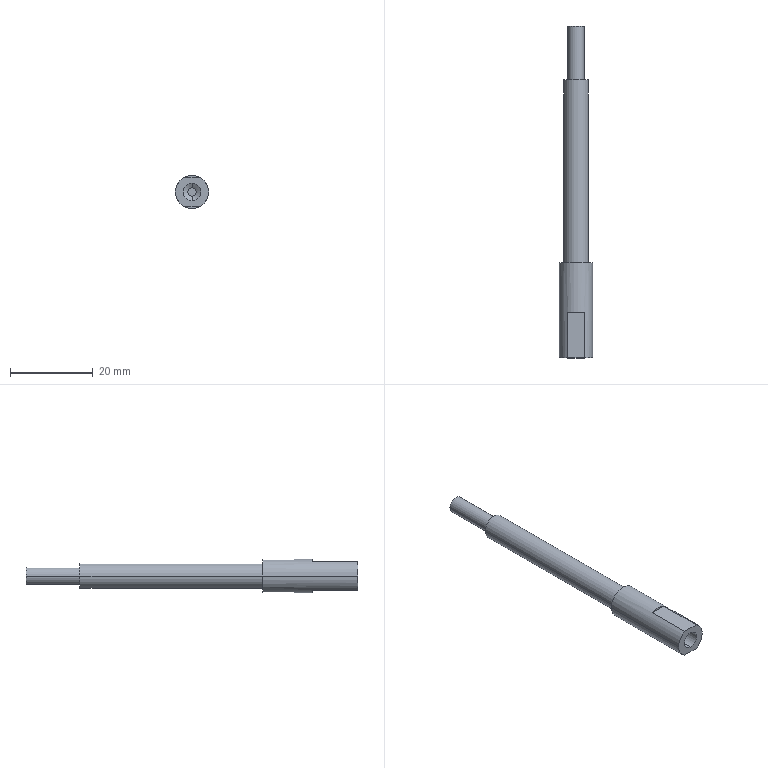Part | SolidWorks | features ICE 4, HoleWzd 1, Revolution 1 | 1 solid | 24 faces | box 8 x 80 x 8 mm | volume 2165 mm3 | cylinder 12 | plane 10 | cone 2 | commonest cylinder face diameters 2 x4 4 x2 4.2 x2 6 x2 8 x2
STEP:
#1=CARTESIAN_POINT('',(-1.,67.,0.));
#2=VERTEX_POINT('',#1);
#3=CARTESIAN_POINT('',(1.,67.,0.));
#4=VERTEX_POINT('',#3);
#5=CARTESIAN_POINT('',(0.,67.,0.));
#6=DIRECTION('',(0.,-1.,0.));
#7=DIRECTION('',(-1.,0.,0.));
#8=AXIS2_PLACEMENT_3D('',#5,#6,#7);
#9=CIRCLE('',#8,1.);
#10=EDGE_CURVE('',#2,#4,#9,.T.);
#11=ORIENTED_EDGE('',*,*,#10,.T.);
#12=CARTESIAN_POINT('',(1.,80.,0.));
#13=VERTEX_POINT('',#12);
#14=CARTESIAN_POINT('',(1.,0.,0.));
#15=DIRECTION('',(0.,1.,0.));
#16=VECTOR('',#15,1000.);
#17=LINE('',#14,#16);
#18=EDGE_CURVE('',#4,#13,#17,.T.);
#19=ORIENTED_EDGE('',*,*,#18,.T.);
#20=CARTESIAN_POINT('',(-1.,80.,0.));
#21=VERTEX_POINT('',#20);
#22=CARTESIAN_POINT('',(0.,80.,0.));
#23=DIRECTION('',(0.,1.,0.));
#24=DIRECTION('',(-1.,0.,0.));
#25=AXIS2_PLACEMENT_3D('',#22,#23,#24);
#26=CIRCLE('',#25,1.);
#27=EDGE_CURVE('',#13,#21,#26,.T.);
#28=ORIENTED_EDGE('',*,*,#27,.T.);
#29=CARTESIAN_POINT('',(-1.,0.,0.));
#30=DIRECTION('',(0.,1.,0.));
#31=VECTOR('',#30,1000.);
#32=LINE('',#29,#31);
#33=EDGE_CURVE('',#2,#21,#32,.T.);
#34=ORIENTED_EDGE('',*,*,#33,.F.);
#35=EDGE_LOOP('',(#11,#19,#28,#34));
#36=FACE_OUTER_BOUND('',#35,.T.);
#37=CARTESIAN_POINT('',(0.,0.,0.));
#38=DIRECTION('',(0.,1.,0.));
#39=DIRECTION('',(-1.,0.,0.));
#40=AXIS2_PLACEMENT_3D('',#37,#38,#39);
#41=CYLINDRICAL_SURFACE('',#40,1.);
#42=ADVANCED_FACE('',(#36),#41,.F.);
#43=CARTESIAN_POINT('',(-2.,67.,0.));
#44=VERTEX_POINT('',#43);
#45=CARTESIAN_POINT('',(2.,67.,0.));
#46=VERTEX_POINT('',#45);
#47=CARTESIAN_POINT('',(0.,67.,0.));
#48=DIRECTION('',(0.,1.,0.));
#49=DIRECTION('',(-1.,0.,0.));
#50=AXIS2_PLACEMENT_3D('',#47,#48,#49);
#51=CIRCLE('',#50,2.);
#52=EDGE_CURVE('',#44,#46,#51,.T.);
#53=ORIENTED_EDGE('',*,*,#52,.T.);
#54=CARTESIAN_POINT('',(2.,80.,0.));
#55=VERTEX_POINT('',#54);
#56=CARTESIAN_POINT('',(2.,80.,0.));
#57=DIRECTION('',(0.,1.,0.));
#58=VECTOR('',#57,1000.);
#59=LINE('',#56,#58);
#60=EDGE_CURVE('',#46,#55,#59,.T.);
#61=ORIENTED_EDGE('',*,*,#60,.T.);
#62=CARTESIAN_POINT('',(-2.,80.,0.));
#63=VERTEX_POINT('',#62);
#64=CARTESIAN_POINT('',(0.,80.,0.));
#65=DIRECTION('',(0.,1.,0.));
#66=DIRECTION('',(-1.,0.,0.));
#67=AXIS2_PLACEMENT_3D('',#64,#65,#66);
#68=CIRCLE('',#67,2.);
#69=EDGE_CURVE('',#63,#55,#68,.T.);
#70=ORIENTED_EDGE('',*,*,#69,.F.);
#71=CARTESIAN_POINT('',(-2.,80.,0.));
#72=DIRECTION('',(0.,1.,0.));
#73=VECTOR('',#72,1000.);
#74=LINE('',#71,#73);
#75=EDGE_CURVE('',#44,#63,#74,.T.);
#76=ORIENTED_EDGE('',*,*,#75,.F.);
#77=EDGE_LOOP('',(#53,#61,#70,#76));
#78=FACE_OUTER_BOUND('',#77,.T.);
#79=CARTESIAN_POINT('',(0.,80.,0.));
#80=DIRECTION('',(0.,1.,0.));
#81=DIRECTION('',(-1.,0.,0.));
#82=AXIS2_PLACEMENT_3D('',#79,#80,#81);
#83=CYLINDRICAL_SURFACE('',#82,2.);
#84=ADVANCED_FACE('',(#78),#83,.T.);
#85=CARTESIAN_POINT('',(0.,12.25,2.1));
#86=VERTEX_POINT('',#85);
#87=CARTESIAN_POINT('',(0.,12.25,-2.1));
#88=VERTEX_POINT('',#87);
#89=CARTESIAN_POINT('',(0.,12.25,0.));
#90=DIRECTION('',(0.,-1.,0.));
#91=DIRECTION('',(0.,0.,-1.));
#92=AXIS2_PLACEMENT_3D('',#89,#90,#91);
#93=CIRCLE('',#92,2.1);
#94=EDGE_CURVE('',#86,#88,#93,.T.);
#95=ORIENTED_EDGE('',*,*,#94,.F.);
#96=CARTESIAN_POINT('',(0.,0.,2.1));
#97=VERTEX_POINT('',#96);
#98=CARTESIAN_POINT('',(0.,0.,2.1));
#99=DIRECTION('',(0.,-1.,0.));
#100=VECTOR('',#99,1000.);
#101=LINE('',#98,#100);
#102=EDGE_CURVE('',#86,#97,#101,.T.);
#103=ORIENTED_EDGE('',*,*,#102,.T.);
#104=CARTESIAN_POINT('',(0.,0.,-2.1));
#105=VERTEX_POINT('',#104);
#106=CARTESIAN_POINT('',(0.,0.,0.));
#107=DIRECTION('',(0.,-1.,0.));
#108=DIRECTION('',(0.,0.,-1.));
#109=AXIS2_PLACEMENT_3D('',#106,#107,#108);
#110=CIRCLE('',#109,2.1);
#111=EDGE_CURVE('',#97,#105,#110,.T.);
#112=ORIENTED_EDGE('',*,*,#111,.T.);
#113=CARTESIAN_POINT('',(0.,0.,-2.1));
#114=DIRECTION('',(0.,-1.,0.));
#115=VECTOR('',#114,1000.);
#116=LINE('',#113,#115);
#117=EDGE_CURVE('',#88,#105,#116,.T.);
#118=ORIENTED_EDGE('',*,*,#117,.F.);
#119=EDGE_LOOP('',(#95,#103,#112,#118));
#120=FACE_OUTER_BOUND('',#119,.T.);
#121=CARTESIAN_POINT('',(0.,0.,0.));
#122=DIRECTION('',(0.,-1.,0.));
#123=DIRECTION('',(0.,0.,-1.));
#124=AXIS2_PLACEMENT_3D('',#121,#122,#123);
#125=CYLINDRICAL_SURFACE('',#124,2.1);
#126=ADVANCED_FACE('',(#120),#125,.F.);
#127=CARTESIAN_POINT('',(0.,12.911,1.));
#128=VERTEX_POINT('',#127);
#129=CARTESIAN_POINT('',(-1.,12.911,0.));
#130=VERTEX_POINT('',#129);
#131=CARTESIAN_POINT('',(0.,12.911,0.));
#132=DIRECTION('',(0.,-1.,0.));
#133=DIRECTION('',(0.,0.,-1.));
#134=AXIS2_PLACEMENT_3D('',#131,#132,#133);
#135=CIRCLE('',#134,1.);
#136=EDGE_CURVE('',#128,#130,#135,.T.);
#137=ORIENTED_EDGE('',*,*,#136,.F.);
#138=CARTESIAN_POINT('',(0.,12.25,2.1));
#139=DIRECTION('',(0.,-0.515,0.8572));
#140=VECTOR('',#139,1000.);
#141=LINE('',#138,#140);
#142=EDGE_CURVE('',#128,#86,#141,.T.);
#143=ORIENTED_EDGE('',*,*,#142,.T.);
#144=ORIENTED_EDGE('',*,*,#94,.T.);
#145=CARTESIAN_POINT('',(0.,12.911,-1.));
#146=VERTEX_POINT('',#145);
#147=CARTESIAN_POINT('',(0.,12.25,-2.1));
#148=DIRECTION('',(0.,-0.515,-0.8572));
#149=VECTOR('',#148,1000.);
#150=LINE('',#147,#149);
#151=EDGE_CURVE('',#146,#88,#150,.T.);
#152=ORIENTED_EDGE('',*,*,#151,.F.);
#153=CARTESIAN_POINT('',(0.,12.911,0.));
#154=DIRECTION('',(0.,-1.,0.));
#155=DIRECTION('',(0.,0.,-1.));
#156=AXIS2_PLACEMENT_3D('',#153,#154,#155);
#157=CIRCLE('',#156,1.);
#158=EDGE_CURVE('',#130,#146,#157,.T.);
#159=ORIENTED_EDGE('',*,*,#158,.F.);
#160=EDGE_LOOP('',(#137,#143,#144,#152,#159));
#161=FACE_OUTER_BOUND('',#160,.T.);
#162=CARTESIAN_POINT('',(0.,12.25,0.));
#163=DIRECTION('',(0.,-1.,0.));
#164=DIRECTION('',(0.,0.,-1.));
#165=AXIS2_PLACEMENT_3D('',#162,#163,#164);
#166=CONICAL_SURFACE('',#165,2.1,1.03);
#167=ADVANCED_FACE('',(#161),#166,.F.);
#168=CARTESIAN_POINT('',(-3.,23.,0.));
#169=VERTEX_POINT('',#168);
#170=CARTESIAN_POINT('',(3.,23.,0.));
#171=VERTEX_POINT('',#170);
#172=CARTESIAN_POINT('',(0.,23.,0.));
#173=DIRECTION('',(0.,1.,0.));
#174=DIRECTION('',(-1.,0.,0.));
#175=AXIS2_PLACEMENT_3D('',#172,#173,#174);
#176=CIRCLE('',#175,3.);
#177=EDGE_CURVE('',#169,#171,#176,.T.);
#178=ORIENTED_EDGE('',*,*,#177,.T.);
#179=CARTESIAN_POINT('',(3.,67.,0.));
#180=VERTEX_POINT('',#179);
#181=CARTESIAN_POINT('',(3.,80.,0.));
#182=DIRECTION('',(0.,1.,0.));
#183=VECTOR('',#182,1000.);
#184=LINE('',#181,#183);
#185=EDGE_CURVE('',#171,#180,#184,.T.);
#186=ORIENTED_EDGE('',*,*,#185,.T.);
#187=CARTESIAN_POINT('',(-3.,67.,0.));
#188=VERTEX_POINT('',#187);
#189=CARTESIAN_POINT('',(0.,67.,0.));
#190=DIRECTION('',(0.,1.,0.));
#191=DIRECTION('',(-1.,0.,0.));
#192=AXIS2_PLACEMENT_3D('',#189,#190,#191);
#193=CIRCLE('',#192,3.);
#194=EDGE_CURVE('',#188,#180,#193,.T.);
#195=ORIENTED_EDGE('',*,*,#194,.F.);
#196=CARTESIAN_POINT('',(-3.,80.,0.));
#197=DIRECTION('',(0.,1.,0.));
#198=VECTOR('',#197,1000.);
#199=LINE('',#196,#198);
#200=EDGE_CURVE('',#169,#188,#199,.T.);
#201=ORIENTED_EDGE('',*,*,#200,.F.);
#202=EDGE_LOOP('',(#178,#186,#195,#201));
#203=FACE_OUTER_BOUND('',#202,.T.);
#204=CARTESIAN_POINT('',(0.,80.,0.));
#205=DIRECTION('',(0.,1.,0.));
#206=DIRECTION('',(-1.,0.,0.));
#207=AXIS2_PLACEMENT_3D('',#204,#205,#206);
#208=CYLINDRICAL_SURFACE('',#207,3.);
#209=ADVANCED_FACE('',(#203),#208,.T.);
#210=CARTESIAN_POINT('',(1.936,0.,3.5));
#211=VERTEX_POINT('',#210);
#212=CARTESIAN_POINT('',(4.,0.,0.));
#213=VERTEX_POINT('',#212);
#214=CARTESIAN_POINT('',(0.,0.,0.));
#215=DIRECTION('',(0.,1.,0.));
#216=DIRECTION('',(-1.,0.,0.));
#217=AXIS2_PLACEMENT_3D('',#214,#215,#216);
#218=CIRCLE('',#217,4.);
#219=EDGE_CURVE('',#211,#213,#218,.T.);
#220=ORIENTED_EDGE('',*,*,#219,.T.);
#221=CARTESIAN_POINT('',(4.,23.,0.));
#222=VERTEX_POINT('',#221);
#223=CARTESIAN_POINT('',(4.,80.,0.));
#224=DIRECTION('',(0.,1.,0.));
#225=VECTOR('',#224,1000.);
#226=LINE('',#223,#225);
#227=EDGE_CURVE('',#213,#222,#226,.T.);
#228=ORIENTED_EDGE('',*,*,#227,.T.);
#229=CARTESIAN_POINT('',(-4.,23.,0.));
#230=VERTEX_POINT('',#229);
#231=CARTESIAN_POINT('',(0.,23.,0.));
#232=DIRECTION('',(0.,1.,0.));
#233=DIRECTION('',(-1.,0.,0.));
#234=AXIS2_PLACEMENT_3D('',#231,#232,#233);
#235=CIRCLE('',#234,4.);
#236=EDGE_CURVE('',#230,#222,#235,.T.);
#237=ORIENTED_EDGE('',*,*,#236,.F.);
#238=CARTESIAN_POINT('',(-4.,0.,0.));
#239=VERTEX_POINT('',#238);
#240=CARTESIAN_POINT('',(-4.,80.,0.));
#241=DIRECTION('',(0.,1.,0.));
#242=VECTOR('',#241,1000.);
#243=LINE('',#240,#242);
#244=EDGE_CURVE('',#239,#230,#243,.T.);
#245=ORIENTED_EDGE('',*,*,#244,.F.);
#246=CARTESIAN_POINT('',(-1.936,0.,3.5));
#247=VERTEX_POINT('',#246);
#248=CARTESIAN_POINT('',(0.,0.,0.));
#249=DIRECTION('',(0.,1.,0.));
#250=DIRECTION('',(-1.,0.,0.));
#251=AXIS2_PLACEMENT_3D('',#248,#249,#250);
#252=CIRCLE('',#251,4.);
#253=EDGE_CURVE('',#239,#247,#252,.T.);
#254=ORIENTED_EDGE('',*,*,#253,.T.);
#255=CARTESIAN_POINT('',(-1.936,11.,3.5));
#256=VERTEX_POINT('',#255);
#257=CARTESIAN_POINT('',(-1.936,80.,3.5));
#258=DIRECTION('',(0.,1.,0.));
#259=VECTOR('',#258,1000.);
#260=LINE('',#257,#259);
#261=EDGE_CURVE('',#247,#256,#260,.T.);
#262=ORIENTED_EDGE('',*,*,#261,.T.);
#263=CARTESIAN_POINT('',(1.936,11.,3.5));
#264=VERTEX_POINT('',#263);
#265=CARTESIAN_POINT('',(0.,11.,0.));
#266=DIRECTION('',(0.,1.,0.));
#267=DIRECTION('',(0.,0.,1.));
#268=AXIS2_PLACEMENT_3D('',#265,#266,#267);
#269=CIRCLE('',#268,4.);
#270=EDGE_CURVE('',#256,#264,#269,.T.);
#271=ORIENTED_EDGE('',*,*,#270,.T.);
#272=CARTESIAN_POINT('',(1.936,80.,3.5));
#273=DIRECTION('',(0.,-1.,0.));
#274=VECTOR('',#273,1000.);
#275=LINE('',#272,#274);
#276=EDGE_CURVE('',#264,#211,#275,.T.);
#277=ORIENTED_EDGE('',*,*,#276,.T.);
#278=EDGE_LOOP('',(#220,#228,#237,#245,#254,#262,#271,#277));
#279=FACE_OUTER_BOUND('',#278,.T.);
#280=CARTESIAN_POINT('',(0.,80.,0.));
#281=DIRECTION('',(0.,1.,0.));
#282=DIRECTION('',(-1.,0.,0.));
#283=AXIS2_PLACEMENT_3D('',#280,#281,#282);
#284=CYLINDRICAL_SURFACE('',#283,4.);
#285=ADVANCED_FACE('',(#279),#284,.T.);
#286=ORIENTED_EDGE('',*,*,#158,.T.);
#287=CARTESIAN_POINT('',(1.,12.911,0.));
#288=VERTEX_POINT('',#287);
#289=CARTESIAN_POINT('',(0.,12.911,0.));
#290=DIRECTION('',(0.,-1.,0.));
#291=DIRECTION('',(0.,0.,-1.));
#292=AXIS2_PLACEMENT_3D('',#289,#290,#291);
#293=CIRCLE('',#292,1.);
#294=EDGE_CURVE('',#146,#288,#293,.T.);
#295=ORIENTED_EDGE('',*,*,#294,.T.);
#296=CARTESIAN_POINT('',(1.,62.,0.));
#297=VERTEX_POINT('',#296);
#298=CARTESIAN_POINT('',(1.,0.,0.));
#299=DIRECTION('',(0.,1.,0.));
#300=VECTOR('',#299,1000.);
#301=LINE('',#298,#300);
#302=EDGE_CURVE('',#288,#297,#301,.T.);
#303=ORIENTED_EDGE('',*,*,#302,.T.);
#304=CARTESIAN_POINT('',(-1.,62.,0.));
#305=VERTEX_POINT('',#304);
#306=CARTESIAN_POINT('',(0.,62.,0.));
#307=DIRECTION('',(0.,-1.,0.));
#308=DIRECTION('',(-1.,0.,0.));
#309=AXIS2_PLACEMENT_3D('',#306,#307,#308);
#310=CIRCLE('',#309,1.);
#311=EDGE_CURVE('',#305,#297,#310,.T.);
#312=ORIENTED_EDGE('',*,*,#311,.F.);
#313=CARTESIAN_POINT('',(-1.,0.,0.));
#314=DIRECTION('',(0.,1.,0.));
#315=VECTOR('',#314,1000.);
#316=LINE('',#313,#315);
#317=EDGE_CURVE('',#130,#305,#316,.T.);
#318=ORIENTED_EDGE('',*,*,#317,.F.);
#319=EDGE_LOOP('',(#286,#295,#303,#312,#318));
#320=FACE_OUTER_BOUND('',#319,.T.);
#321=CARTESIAN_POINT('',(0.,0.,0.));
#322=DIRECTION('',(0.,1.,0.));
#323=DIRECTION('',(-1.,0.,0.));
#324=AXIS2_PLACEMENT_3D('',#321,#322,#323);
#325=CYLINDRICAL_SURFACE('',#324,1.);
#326=ADVANCED_FACE('',(#320),#325,.F.);
#327=ORIENTED_EDGE('',*,*,#302,.F.);
#328=CARTESIAN_POINT('',(0.,12.911,0.));
#329=DIRECTION('',(0.,-1.,0.));
#330=DIRECTION('',(0.,0.,-1.));
#331=AXIS2_PLACEMENT_3D('',#328,#329,#330);
#332=CIRCLE('',#331,1.);
#333=EDGE_CURVE('',#288,#128,#332,.T.);
#334=ORIENTED_EDGE('',*,*,#333,.T.);
#335=ORIENTED_EDGE('',*,*,#136,.T.);
#336=ORIENTED_EDGE('',*,*,#317,.T.);
#337=CARTESIAN_POINT('',(0.,62.,0.));
#338=DIRECTION('',(0.,-1.,0.));
#339=DIRECTION('',(-1.,0.,0.));
#340=AXIS2_PLACEMENT_3D('',#337,#338,#339);
#341=CIRCLE('',#340,1.);
#342=EDGE_CURVE('',#297,#305,#341,.T.);
#343=ORIENTED_EDGE('',*,*,#342,.F.);
#344=EDGE_LOOP('',(#327,#334,#335,#336,#343));
#345=FACE_OUTER_BOUND('',#344,.T.);
#346=CARTESIAN_POINT('',(0.,0.,0.));
#347=DIRECTION('',(0.,1.,0.));
#348=DIRECTION('',(-1.,0.,0.));
#349=AXIS2_PLACEMENT_3D('',#346,#347,#348);
#350=CYLINDRICAL_SURFACE('',#349,1.);
#351=ADVANCED_FACE('',(#345),#350,.F.);
#352=ORIENTED_EDGE('',*,*,#227,.F.);
#353=CARTESIAN_POINT('',(1.936,0.,-3.5));
#354=VERTEX_POINT('',#353);
#355=CARTESIAN_POINT('',(0.,0.,0.));
#356=DIRECTION('',(0.,1.,0.));
#357=DIRECTION('',(-1.,0.,0.));
#358=AXIS2_PLACEMENT_3D('',#355,#356,#357);
#359=CIRCLE('',#358,4.);
#360=EDGE_CURVE('',#213,#354,#359,.T.);
#361=ORIENTED_EDGE('',*,*,#360,.T.);
#362=CARTESIAN_POINT('',(1.936,11.,-3.5));
#363=VERTEX_POINT('',#362);
#364=CARTESIAN_POINT('',(1.936,80.,-3.5));
#365=DIRECTION('',(0.,1.,0.));
#366=VECTOR('',#365,1000.);
#367=LINE('',#364,#366);
#368=EDGE_CURVE('',#354,#363,#367,.T.);
#369=ORIENTED_EDGE('',*,*,#368,.T.);
#370=CARTESIAN_POINT('',(-1.936,11.,-3.5));
#371=VERTEX_POINT('',#370);
#372=CARTESIAN_POINT('',(0.,11.,0.));
#373=DIRECTION('',(0.,1.,0.));
#374=DIRECTION('',(0.,0.,1.));
#375=AXIS2_PLACEMENT_3D('',#372,#373,#374);
#376=CIRCLE('',#375,4.);
#377=EDGE_CURVE('',#363,#371,#376,.T.);
#378=ORIENTED_EDGE('',*,*,#377,.T.);
#379=CARTESIAN_POINT('',(-1.936,0.,-3.5));
#380=VERTEX_POINT('',#379);
#381=CARTESIAN_POINT('',(-1.936,80.,-3.5));
#382=DIRECTION('',(0.,-1.,0.));
#383=VECTOR('',#382,1000.);
#384=LINE('',#381,#383);
#385=EDGE_CURVE('',#371,#380,#384,.T.);
#386=ORIENTED_EDGE('',*,*,#385,.T.);
#387=CARTESIAN_POINT('',(0.,0.,0.));
#388=DIRECTION('',(0.,1.,0.));
#389=DIRECTION('',(-1.,0.,0.));
#390=AXIS2_PLACEMENT_3D('',#387,#388,#389);
#391=CIRCLE('',#390,4.);
#392=EDGE_CURVE('',#380,#239,#391,.T.);
#393=ORIENTED_EDGE('',*,*,#392,.T.);
#394=ORIENTED_EDGE('',*,*,#244,.T.);
#395=CARTESIAN_POINT('',(0.,23.,0.));
#396=DIRECTION('',(0.,1.,0.));
#397=DIRECTION('',(-1.,0.,0.));
#398=AXIS2_PLACEMENT_3D('',#395,#396,#397);
#399=CIRCLE('',#398,4.);
#400=EDGE_CURVE('',#222,#230,#399,.T.);
#401=ORIENTED_EDGE('',*,*,#400,.F.);
#402=EDGE_LOOP('',(#352,#361,#369,#378,#386,#393,#394,#401));
#403=FACE_OUTER_BOUND('',#402,.T.);
#404=CARTESIAN_POINT('',(0.,80.,0.));
#405=DIRECTION('',(0.,1.,0.));
#406=DIRECTION('',(-1.,0.,0.));
#407=AXIS2_PLACEMENT_3D('',#404,#405,#406);
#408=CYLINDRICAL_SURFACE('',#407,4.);
#409=ADVANCED_FACE('',(#403),#408,.T.);
#410=ORIENTED_EDGE('',*,*,#177,.F.);
#411=CARTESIAN_POINT('',(0.,23.,0.));
#412=DIRECTION('',(0.,1.,0.));
#413=DIRECTION('',(-1.,0.,0.));
#414=AXIS2_PLACEMENT_3D('',#411,#412,#413);
#415=CIRCLE('',#414,3.);
#416=EDGE_CURVE('',#171,#169,#415,.T.);
#417=ORIENTED_EDGE('',*,*,#416,.F.);
#418=EDGE_LOOP('',(#410,#417));
#419=FACE_BOUND('',#418,.T.);
#420=ORIENTED_EDGE('',*,*,#236,.T.);
#421=ORIENTED_EDGE('',*,*,#400,.T.);
#422=EDGE_LOOP('',(#420,#421));
#423=FACE_OUTER_BOUND('',#422,.T.);
#424=CARTESIAN_POINT('',(3.,23.,0.));
#425=DIRECTION('',(0.,-1.,0.));
#426=DIRECTION('',(1.,0.,0.));
#427=AXIS2_PLACEMENT_3D('',#424,#425,#426);
#428=PLANE('',#427);
#429=ADVANCED_FACE('',(#419,#423),#428,.F.);
#430=ORIENTED_EDGE('',*,*,#185,.F.);
#431=ORIENTED_EDGE('',*,*,#416,.T.);
#432=ORIENTED_EDGE('',*,*,#200,.T.);
#433=CARTESIAN_POINT('',(0.,67.,0.));
#434=DIRECTION('',(0.,1.,0.));
#435=DIRECTION('',(-1.,0.,0.));
#436=AXIS2_PLACEMENT_3D('',#433,#434,#435);
#437=CIRCLE('',#436,3.);
#438=EDGE_CURVE('',#180,#188,#437,.T.);
#439=ORIENTED_EDGE('',*,*,#438,.F.);
#440=EDGE_LOOP('',(#430,#431,#432,#439));
#441=FACE_OUTER_BOUND('',#440,.T.);
#442=CARTESIAN_POINT('',(0.,80.,0.));
#443=DIRECTION('',(0.,1.,0.));
#444=DIRECTION('',(-1.,0.,0.));
#445=AXIS2_PLACEMENT_3D('',#442,#443,#444);
#446=CYLINDRICAL_SURFACE('',#445,3.);
#447=ADVANCED_FACE('',(#441),#446,.T.);
#448=CARTESIAN_POINT('',(0.,0.,0.));
#449=DIRECTION('',(0.,-1.,0.));
#450=DIRECTION('',(0.,0.,-1.));
#451=AXIS2_PLACEMENT_3D('',#448,#449,#450);
#452=CIRCLE('',#451,2.1);
#453=EDGE_CURVE('',#105,#97,#452,.T.);
#454=ORIENTED_EDGE('',*,*,#453,.F.);
#455=ORIENTED_EDGE('',*,*,#111,.F.);
#456=EDGE_LOOP('',(#454,#455));
#457=FACE_BOUND('',#456,.T.);
#458=ORIENTED_EDGE('',*,*,#219,.F.);
#459=CARTESIAN_POINT('',(0.,0.,3.5));
#460=DIRECTION('',(-1.,0.,0.));
#461=VECTOR('',#460,1000.);
#462=LINE('',#459,#461);
#463=EDGE_CURVE('',#211,#247,#462,.T.);
#464=ORIENTED_EDGE('',*,*,#463,.T.);
#465=ORIENTED_EDGE('',*,*,#253,.F.);
#466=ORIENTED_EDGE('',*,*,#392,.F.);
#467=CARTESIAN_POINT('',(0.,0.,-3.5));
#468=DIRECTION('',(1.,0.,0.));
#469=VECTOR('',#468,1000.);
#470=LINE('',#467,#469);
#471=EDGE_CURVE('',#380,#354,#470,.T.);
#472=ORIENTED_EDGE('',*,*,#471,.T.);
#473=ORIENTED_EDGE('',*,*,#360,.F.);
#474=EDGE_LOOP('',(#458,#464,#465,#466,#472,#473));
#475=FACE_OUTER_BOUND('',#474,.T.);
#476=CARTESIAN_POINT('',(0.,0.,0.));
#477=DIRECTION('',(0.,1.,0.));
#478=DIRECTION('',(-1.,0.,0.));
#479=AXIS2_PLACEMENT_3D('',#476,#477,#478);
#480=PLANE('',#479);
#481=ADVANCED_FACE('',(#457,#475),#480,.F.);
#482=ORIENTED_EDGE('',*,*,#142,.F.);
#483=ORIENTED_EDGE('',*,*,#333,.F.);
#484=ORIENTED_EDGE('',*,*,#294,.F.);
#485=ORIENTED_EDGE('',*,*,#151,.T.);
#486=CARTESIAN_POINT('',(0.,12.25,0.));
#487=DIRECTION('',(0.,-1.,0.));
#488=DIRECTION('',(0.,0.,-1.));
#489=AXIS2_PLACEMENT_3D('',#486,#487,#488);
#490=CIRCLE('',#489,2.1);
#491=EDGE_CURVE('',#88,#86,#490,.T.);
#492=ORIENTED_EDGE('',*,*,#491,.T.);
#493=EDGE_LOOP('',(#482,#483,#484,#485,#492));
#494=FACE_OUTER_BOUND('',#493,.T.);
#495=CARTESIAN_POINT('',(0.,12.25,0.));
#496=DIRECTION('',(0.,-1.,0.));
#497=DIRECTION('',(0.,0.,-1.));
#498=AXIS2_PLACEMENT_3D('',#495,#496,#497);
#499=CONICAL_SURFACE('',#498,2.1,1.03);
#500=ADVANCED_FACE('',(#494),#499,.F.);
#501=ORIENTED_EDGE('',*,*,#102,.F.);
#502=ORIENTED_EDGE('',*,*,#491,.F.);
#503=ORIENTED_EDGE('',*,*,#117,.T.);
#504=ORIENTED_EDGE('',*,*,#453,.T.);
#505=EDGE_LOOP('',(#501,#502,#503,#504));
#506=FACE_OUTER_BOUND('',#505,.T.);
#507=CARTESIAN_POINT('',(0.,0.,0.));
#508=DIRECTION('',(0.,-1.,0.));
#509=DIRECTION('',(0.,0.,-1.));
#510=AXIS2_PLACEMENT_3D('',#507,#508,#509);
#511=CYLINDRICAL_SURFACE('',#510,2.1);
#512=ADVANCED_FACE('',(#506),#511,.F.);
#513=CARTESIAN_POINT('',(-4.,11.,-3.5));
#514=DIRECTION('',(1.,0.,0.));
#515=VECTOR('',#514,1000.);
#516=LINE('',#513,#515);
#517=EDGE_CURVE('',#371,#363,#516,.T.);
#518=ORIENTED_EDGE('',*,*,#517,.F.);
#519=ORIENTED_EDGE('',*,*,#377,.F.);
#520=EDGE_LOOP('',(#518,#519));
#521=FACE_OUTER_BOUND('',#520,.T.);
#522=CARTESIAN_POINT('',(-4.,11.,-5.928));
#523=DIRECTION('',(0.,1.,0.));
#524=DIRECTION('',(0.,0.,1.));
#525=AXIS2_PLACEMENT_3D('',#522,#523,#524);
#526=PLANE('',#525);
#527=ADVANCED_FACE('',(#521),#526,.F.);
#528=ORIENTED_EDGE('',*,*,#471,.F.);
#529=ORIENTED_EDGE('',*,*,#385,.F.);
#530=ORIENTED_EDGE('',*,*,#517,.T.);
#531=ORIENTED_EDGE('',*,*,#368,.F.);
#532=EDGE_LOOP('',(#528,#529,#530,#531));
#533=FACE_OUTER_BOUND('',#532,.T.);
#534=CARTESIAN_POINT('',(-4.,11.,-3.5));
#535=DIRECTION('',(0.,0.,1.));
#536=DIRECTION('',(0.,-1.,0.));
#537=AXIS2_PLACEMENT_3D('',#534,#535,#536);
#538=PLANE('',#537);
#539=ADVANCED_FACE('',(#533),#538,.F.);
#540=CARTESIAN_POINT('',(-4.,11.,3.5));
#541=DIRECTION('',(1.,0.,0.));
#542=VECTOR('',#541,1000.);
#543=LINE('',#540,#542);
#544=EDGE_CURVE('',#256,#264,#543,.T.);
#545=ORIENTED_EDGE('',*,*,#544,.T.);
#546=ORIENTED_EDGE('',*,*,#270,.F.);
#547=EDGE_LOOP('',(#545,#546));
#548=FACE_OUTER_BOUND('',#547,.T.);
#549=CARTESIAN_POINT('',(-4.,11.,7.669));
#550=DIRECTION('',(0.,1.,0.));
#551=DIRECTION('',(0.,0.,1.));
#552=AXIS2_PLACEMENT_3D('',#549,#550,#551);
#553=PLANE('',#552);
#554=ADVANCED_FACE('',(#548),#553,.F.);
#555=ORIENTED_EDGE('',*,*,#463,.F.);
#556=ORIENTED_EDGE('',*,*,#276,.F.);
#557=ORIENTED_EDGE('',*,*,#544,.F.);
#558=ORIENTED_EDGE('',*,*,#261,.F.);
#559=EDGE_LOOP('',(#555,#556,#557,#558));
#560=FACE_OUTER_BOUND('',#559,.T.);
#561=CARTESIAN_POINT('',(-4.,11.,3.5));
#562=DIRECTION('',(0.,0.,-1.));
#563=DIRECTION('',(0.,1.,0.));
#564=AXIS2_PLACEMENT_3D('',#561,#562,#563);
#565=PLANE('',#564);
#566=ADVANCED_FACE('',(#560),#565,.F.);
#567=ORIENTED_EDGE('',*,*,#311,.T.);
#568=ORIENTED_EDGE('',*,*,#342,.T.);
#569=EDGE_LOOP('',(#567,#568));
#570=FACE_OUTER_BOUND('',#569,.T.);
#571=CARTESIAN_POINT('',(0.,62.,0.));
#572=DIRECTION('',(0.,1.,0.));
#573=DIRECTION('',(-1.,0.,0.));
#574=AXIS2_PLACEMENT_3D('',#571,#572,#573);
#575=PLANE('',#574);
#576=ADVANCED_FACE('',(#570),#575,.F.);
#577=ORIENTED_EDGE('',*,*,#194,.T.);
#578=ORIENTED_EDGE('',*,*,#438,.T.);
#579=EDGE_LOOP('',(#577,#578));
#580=FACE_OUTER_BOUND('',#579,.T.);
#581=ORIENTED_EDGE('',*,*,#52,.F.);
#582=CARTESIAN_POINT('',(0.,67.,0.));
#583=DIRECTION('',(0.,1.,0.));
#584=DIRECTION('',(-1.,0.,0.));
#585=AXIS2_PLACEMENT_3D('',#582,#583,#584);
#586=CIRCLE('',#585,2.);
#587=EDGE_CURVE('',#46,#44,#586,.T.);
#588=ORIENTED_EDGE('',*,*,#587,.F.);
#589=EDGE_LOOP('',(#581,#588));
#590=FACE_BOUND('',#589,.T.);
#591=CARTESIAN_POINT('',(0.,67.,0.));
#592=DIRECTION('',(0.,1.,0.));
#593=DIRECTION('',(-1.,0.,0.));
#594=AXIS2_PLACEMENT_3D('',#591,#592,#593);
#595=PLANE('',#594);
#596=ADVANCED_FACE('',(#580,#590),#595,.T.);
#597=ORIENTED_EDGE('',*,*,#60,.F.);
#598=ORIENTED_EDGE('',*,*,#587,.T.);
#599=ORIENTED_EDGE('',*,*,#75,.T.);
#600=CARTESIAN_POINT('',(0.,80.,0.));
#601=DIRECTION('',(0.,1.,0.));
#602=DIRECTION('',(-1.,0.,0.));
#603=AXIS2_PLACEMENT_3D('',#600,#601,#602);
#604=CIRCLE('',#603,2.);
#605=EDGE_CURVE('',#55,#63,#604,.T.);
#606=ORIENTED_EDGE('',*,*,#605,.F.);
#607=EDGE_LOOP('',(#597,#598,#599,#606));
#608=FACE_OUTER_BOUND('',#607,.T.);
#609=CARTESIAN_POINT('',(0.,80.,0.));
#610=DIRECTION('',(0.,1.,0.));
#611=DIRECTION('',(-1.,0.,0.));
#612=AXIS2_PLACEMENT_3D('',#609,#610,#611);
#613=CYLINDRICAL_SURFACE('',#612,2.);
#614=ADVANCED_FACE('',(#608),#613,.T.);
#615=CARTESIAN_POINT('',(0.,80.,0.));
#616=DIRECTION('',(0.,1.,0.));
#617=DIRECTION('',(-1.,0.,0.));
#618=AXIS2_PLACEMENT_3D('',#615,#616,#617);
#619=CIRCLE('',#618,1.);
#620=EDGE_CURVE('',#21,#13,#619,.T.);
#621=ORIENTED_EDGE('',*,*,#620,.F.);
#622=ORIENTED_EDGE('',*,*,#27,.F.);
#623=EDGE_LOOP('',(#621,#622));
#624=FACE_BOUND('',#623,.T.);
#625=ORIENTED_EDGE('',*,*,#69,.T.);
#626=ORIENTED_EDGE('',*,*,#605,.T.);
#627=EDGE_LOOP('',(#625,#626));
#628=FACE_OUTER_BOUND('',#627,.T.);
#629=CARTESIAN_POINT('',(0.,80.,0.));
#630=DIRECTION('',(0.,-1.,0.));
#631=DIRECTION('',(1.,0.,0.));
#632=AXIS2_PLACEMENT_3D('',#629,#630,#631);
#633=PLANE('',#632);
#634=ADVANCED_FACE('',(#624,#628),#633,.F.);
#635=ORIENTED_EDGE('',*,*,#18,.F.);
#636=CARTESIAN_POINT('',(0.,67.,0.));
#637=DIRECTION('',(0.,-1.,0.));
#638=DIRECTION('',(-1.,0.,0.));
#639=AXIS2_PLACEMENT_3D('',#636,#637,#638);
#640=CIRCLE('',#639,1.);
#641=EDGE_CURVE('',#4,#2,#640,.T.);
#642=ORIENTED_EDGE('',*,*,#641,.T.);
#643=ORIENTED_EDGE('',*,*,#33,.T.);
#644=ORIENTED_EDGE('',*,*,#620,.T.);
#645=EDGE_LOOP('',(#635,#642,#643,#644));
#646=FACE_OUTER_BOUND('',#645,.T.);
#647=CARTESIAN_POINT('',(0.,0.,0.));
#648=DIRECTION('',(0.,1.,0.));
#649=DIRECTION('',(-1.,0.,0.));
#650=AXIS2_PLACEMENT_3D('',#647,#648,#649);
#651=CYLINDRICAL_SURFACE('',#650,1.);
#652=ADVANCED_FACE('',(#646),#651,.F.);
#653=ORIENTED_EDGE('',*,*,#10,.F.);
#654=ORIENTED_EDGE('',*,*,#641,.F.);
#655=EDGE_LOOP('',(#653,#654));
#656=FACE_OUTER_BOUND('',#655,.T.);
#657=CARTESIAN_POINT('',(0.,67.,0.));
#658=DIRECTION('',(0.,1.,0.));
#659=DIRECTION('',(-1.,0.,0.));
#660=AXIS2_PLACEMENT_3D('',#657,#658,#659);
#661=PLANE('',#660);
#662=ADVANCED_FACE('',(#656),#661,.T.);
#663=CLOSED_SHELL('',(#42,#84,#126,#167,#209,#285,#326,#351,#409,#429,#447,#481,#500,#512,#527,#539,#554,#566,#576,#596,#614,#634,#652,#662));
#664=MANIFOLD_SOLID_BREP('',#663);
#665=CARTESIAN_POINT('',(0.,0.,0.));
#666=DIRECTION('',(0.,0.,1.));
#667=DIRECTION('',(1.,0.,0.));
#668=AXIS2_PLACEMENT_3D('',#665,#666,#667);
#669=(LENGTH_UNIT()NAMED_UNIT(*)SI_UNIT(.MILLI.,.METRE.));
#670=UNCERTAINTY_MEASURE_WITH_UNIT(LENGTH_MEASURE(0.00001),#669,'','');
#671=(NAMED_UNIT(*)PLANE_ANGLE_UNIT()SI_UNIT($,.RADIAN.));
#672=(NAMED_UNIT(*)SI_UNIT($,.STERADIAN.)SOLID_ANGLE_UNIT());
#673=(GEOMETRIC_REPRESENTATION_CONTEXT(3)GLOBAL_UNCERTAINTY_ASSIGNED_CONTEXT((#670))GLOBAL_UNIT_ASSIGNED_CONTEXT((#669,#671,#672))REPRESENTATION_CONTEXT('',''));
#674=ADVANCED_BREP_SHAPE_REPRESENTATION('',(#664,#668),#673);